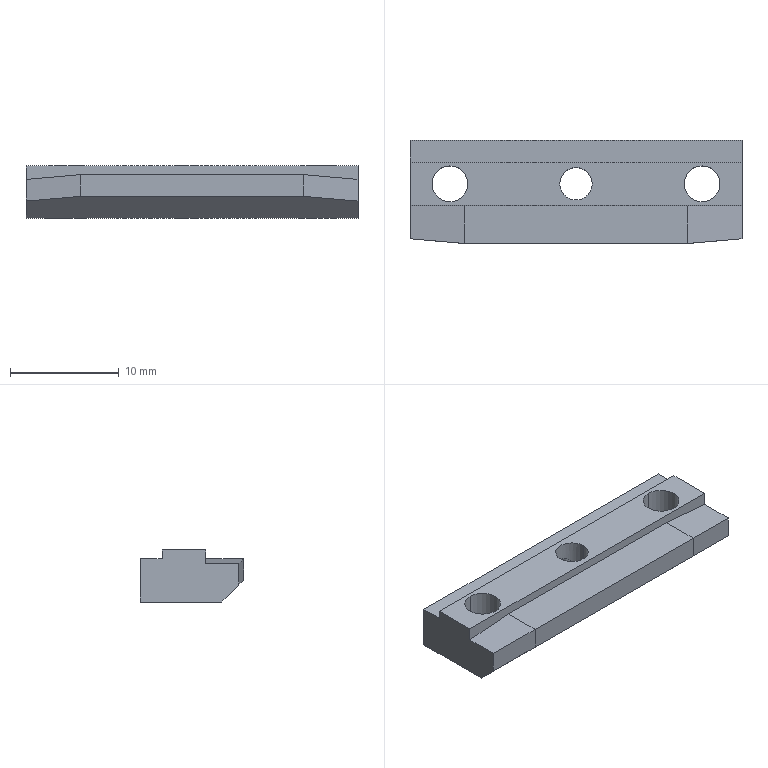Part | NX | 1 solid | 29 faces | box 30.6 x 9.5 x 4.8 mm | volume 1058 mm3 | plane 15 | cylinder 8 | cone 6 | commonest cylinder face diameters 3.3 x4 2.5 x2 3 x2
STEP:
#1=CARTESIAN_POINT('',(-174.8,180.7,-95.7));
#2=VERTEX_POINT('',#1);
#3=CARTESIAN_POINT('',(-174.8,176.706,-95.7));
#4=VERTEX_POINT('',#3);
#5=CARTESIAN_POINT('',(-174.8,178.513,-95.7));
#6=DIRECTION('',(0.,-1.,0.));
#7=VECTOR('',#6,1000.);
#8=LINE('',#5,#7);
#9=EDGE_CURVE('',#2,#4,#8,.T.);
#10=ORIENTED_EDGE('',*,*,#9,.T.);
#11=CARTESIAN_POINT('',(-144.2,176.706,-95.7));
#12=VERTEX_POINT('',#11);
#13=CARTESIAN_POINT('',(-175.,176.706,-95.7));
#14=DIRECTION('',(-1.,0.,0.));
#15=VECTOR('',#14,1000.);
#16=LINE('',#13,#15);
#17=EDGE_CURVE('',#12,#4,#16,.T.);
#18=ORIENTED_EDGE('',*,*,#17,.F.);
#19=CARTESIAN_POINT('',(-144.2,180.7,-95.7));
#20=VERTEX_POINT('',#19);
#21=CARTESIAN_POINT('',(-144.2,178.513,-95.7));
#22=DIRECTION('',(0.,-1.,0.));
#23=VECTOR('',#22,1000.);
#24=LINE('',#21,#23);
#25=EDGE_CURVE('',#20,#12,#24,.T.);
#26=ORIENTED_EDGE('',*,*,#25,.F.);
#27=CARTESIAN_POINT('',(-175.,180.7,-95.7));
#28=DIRECTION('',(1.,0.,0.));
#29=VECTOR('',#28,1000.);
#30=LINE('',#27,#29);
#31=EDGE_CURVE('',#2,#20,#30,.T.);
#32=ORIENTED_EDGE('',*,*,#31,.F.);
#33=EDGE_LOOP('',(#10,#18,#26,#32));
#34=FACE_BOUND('',#33,.T.);
#35=CARTESIAN_POINT('',(-147.875,177.05,-95.7));
#36=VERTEX_POINT('',#35);
#37=CARTESIAN_POINT('',(-147.875,180.35,-95.7));
#38=VERTEX_POINT('',#37);
#39=CARTESIAN_POINT('',(-147.875,178.7,-95.7));
#40=DIRECTION('',(0.,0.,-1.));
#41=DIRECTION('',(0.,1.,0.));
#42=AXIS2_PLACEMENT_3D('',#39,#40,#41);
#43=CIRCLE('',#42,1.65);
#44=EDGE_CURVE('',#36,#38,#43,.T.);
#45=ORIENTED_EDGE('',*,*,#44,.T.);
#46=CARTESIAN_POINT('',(-147.875,178.7,-95.7));
#47=DIRECTION('',(0.,0.,-1.));
#48=DIRECTION('',(0.,1.,0.));
#49=AXIS2_PLACEMENT_3D('',#46,#47,#48);
#50=CIRCLE('',#49,1.65);
#51=EDGE_CURVE('',#38,#36,#50,.T.);
#52=ORIENTED_EDGE('',*,*,#51,.T.);
#53=EDGE_LOOP('',(#45,#52));
#54=FACE_BOUND('',#53,.T.);
#55=CARTESIAN_POINT('',(-171.125,177.05,-95.7));
#56=VERTEX_POINT('',#55);
#57=CARTESIAN_POINT('',(-171.125,180.35,-95.7));
#58=VERTEX_POINT('',#57);
#59=CARTESIAN_POINT('',(-171.125,178.7,-95.7));
#60=DIRECTION('',(0.,0.,-1.));
#61=DIRECTION('',(0.,1.,0.));
#62=AXIS2_PLACEMENT_3D('',#59,#60,#61);
#63=CIRCLE('',#62,1.65);
#64=EDGE_CURVE('',#56,#58,#63,.T.);
#65=ORIENTED_EDGE('',*,*,#64,.T.);
#66=CARTESIAN_POINT('',(-171.125,178.7,-95.7));
#67=DIRECTION('',(0.,0.,-1.));
#68=DIRECTION('',(0.,1.,0.));
#69=AXIS2_PLACEMENT_3D('',#66,#67,#68);
#70=CIRCLE('',#69,1.65);
#71=EDGE_CURVE('',#58,#56,#70,.T.);
#72=ORIENTED_EDGE('',*,*,#71,.T.);
#73=EDGE_LOOP('',(#65,#72));
#74=FACE_BOUND('',#73,.T.);
#75=CARTESIAN_POINT('',(-158.,178.7,-95.7));
#76=VERTEX_POINT('',#75);
#77=CARTESIAN_POINT('',(-161.,178.7,-95.7));
#78=VERTEX_POINT('',#77);
#79=CARTESIAN_POINT('',(-159.5,178.7,-95.7));
#80=DIRECTION('',(0.,0.,-1.));
#81=DIRECTION('',(-1.,0.,0.));
#82=AXIS2_PLACEMENT_3D('',#79,#80,#81);
#83=CIRCLE('',#82,1.5);
#84=EDGE_CURVE('',#76,#78,#83,.T.);
#85=ORIENTED_EDGE('',*,*,#84,.T.);
#86=CARTESIAN_POINT('',(-159.5,178.7,-95.7));
#87=DIRECTION('',(0.,0.,-1.));
#88=DIRECTION('',(-1.,0.,0.));
#89=AXIS2_PLACEMENT_3D('',#86,#87,#88);
#90=CIRCLE('',#89,1.5);
#91=EDGE_CURVE('',#78,#76,#90,.T.);
#92=ORIENTED_EDGE('',*,*,#91,.T.);
#93=EDGE_LOOP('',(#85,#92));
#94=FACE_BOUND('',#93,.T.);
#95=CARTESIAN_POINT('',(-175.,176.707,-95.7));
#96=DIRECTION('',(0.,0.,1.));
#97=DIRECTION('',(1.,0.,0.));
#98=AXIS2_PLACEMENT_3D('',#95,#96,#97);
#99=PLANE('',#98);
#100=ADVANCED_FACE('',(#34,#54,#74,#94),#99,.T.);
#101=CARTESIAN_POINT('',(-174.8,176.697,-96.937));
#102=VERTEX_POINT('',#101);
#103=CARTESIAN_POINT('',(-174.8,176.744,-90.15));
#104=DIRECTION('',(0.,-0.007004,-1.));
#105=VECTOR('',#104,1000.);
#106=LINE('',#103,#105);
#107=EDGE_CURVE('',#4,#102,#106,.T.);
#108=ORIENTED_EDGE('',*,*,#107,.T.);
#109=CARTESIAN_POINT('',(-169.8,176.7,-96.5));
#110=VERTEX_POINT('',#109);
#111=CARTESIAN_POINT('',(-175.,176.697,-96.955));
#112=DIRECTION('',(-0.9962,-0.0006105,-0.08716));
#113=VECTOR('',#112,1000.);
#114=LINE('',#111,#113);
#115=EDGE_CURVE('',#110,#102,#114,.T.);
#116=ORIENTED_EDGE('',*,*,#115,.F.);
#117=CARTESIAN_POINT('',(-149.2,176.7,-96.5));
#118=VERTEX_POINT('',#117);
#119=CARTESIAN_POINT('',(-175.,176.7,-96.5));
#120=DIRECTION('',(1.,0.,0.));
#121=VECTOR('',#120,1000.);
#122=LINE('',#119,#121);
#123=EDGE_CURVE('',#110,#118,#122,.T.);
#124=ORIENTED_EDGE('',*,*,#123,.T.);
#125=CARTESIAN_POINT('',(-144.2,176.697,-96.937));
#126=VERTEX_POINT('',#125);
#127=CARTESIAN_POINT('',(-175.,176.716,-94.243));
#128=DIRECTION('',(0.9962,-0.0006105,-0.08716));
#129=VECTOR('',#128,1000.);
#130=LINE('',#127,#129);
#131=EDGE_CURVE('',#118,#126,#130,.T.);
#132=ORIENTED_EDGE('',*,*,#131,.T.);
#133=CARTESIAN_POINT('',(-144.2,176.744,-90.15));
#134=DIRECTION('',(0.,-0.007004,-1.));
#135=VECTOR('',#134,1000.);
#136=LINE('',#133,#135);
#137=EDGE_CURVE('',#12,#126,#136,.T.);
#138=ORIENTED_EDGE('',*,*,#137,.F.);
#139=ORIENTED_EDGE('',*,*,#17,.T.);
#140=EDGE_LOOP('',(#108,#116,#124,#132,#138,#139));
#141=FACE_BOUND('',#140,.T.);
#142=CARTESIAN_POINT('',(-175.,176.7,-96.5));
#143=DIRECTION('',(0.,-1.,0.007004));
#144=DIRECTION('',(-1.,0.,0.));
#145=AXIS2_PLACEMENT_3D('',#142,#143,#144);
#146=PLANE('',#145);
#147=ADVANCED_FACE('',(#141),#146,.T.);
#148=CARTESIAN_POINT('',(-169.8,173.2,-96.5));
#149=VERTEX_POINT('',#148);
#150=CARTESIAN_POINT('',(-169.8,174.95,-96.5));
#151=DIRECTION('',(0.,-1.,0.));
#152=VECTOR('',#151,1000.);
#153=LINE('',#150,#152);
#154=EDGE_CURVE('',#110,#149,#153,.T.);
#155=ORIENTED_EDGE('',*,*,#154,.T.);
#156=CARTESIAN_POINT('',(-149.2,173.2,-96.5));
#157=VERTEX_POINT('',#156);
#158=CARTESIAN_POINT('',(-175.,173.2,-96.5));
#159=DIRECTION('',(1.,0.,0.));
#160=VECTOR('',#159,1000.);
#161=LINE('',#158,#160);
#162=EDGE_CURVE('',#149,#157,#161,.T.);
#163=ORIENTED_EDGE('',*,*,#162,.T.);
#164=CARTESIAN_POINT('',(-149.2,174.95,-96.5));
#165=DIRECTION('',(0.,-1.,0.));
#166=VECTOR('',#165,1000.);
#167=LINE('',#164,#166);
#168=EDGE_CURVE('',#118,#157,#167,.T.);
#169=ORIENTED_EDGE('',*,*,#168,.F.);
#170=ORIENTED_EDGE('',*,*,#123,.F.);
#171=EDGE_LOOP('',(#155,#163,#169,#170));
#172=FACE_BOUND('',#171,.T.);
#173=CARTESIAN_POINT('',(-175.,174.7,-96.5));
#174=DIRECTION('',(0.,0.,1.));
#175=DIRECTION('',(1.,0.,0.));
#176=AXIS2_PLACEMENT_3D('',#173,#174,#175);
#177=PLANE('',#176);
#178=ADVANCED_FACE('',(#172),#177,.T.);
#179=CARTESIAN_POINT('',(-149.2,173.2,-98.5));
#180=VERTEX_POINT('',#179);
#181=CARTESIAN_POINT('',(-169.8,173.2,-98.5));
#182=VERTEX_POINT('',#181);
#183=CARTESIAN_POINT('',(-175.,173.2,-98.5));
#184=DIRECTION('',(-1.,0.,0.));
#185=VECTOR('',#184,1000.);
#186=LINE('',#183,#185);
#187=EDGE_CURVE('',#180,#182,#186,.T.);
#188=ORIENTED_EDGE('',*,*,#187,.F.);
#189=CARTESIAN_POINT('',(-149.2,173.2,-97.5));
#190=DIRECTION('',(0.,0.,-1.));
#191=VECTOR('',#190,1000.);
#192=LINE('',#189,#191);
#193=EDGE_CURVE('',#157,#180,#192,.T.);
#194=ORIENTED_EDGE('',*,*,#193,.F.);
#195=ORIENTED_EDGE('',*,*,#162,.F.);
#196=CARTESIAN_POINT('',(-169.8,173.2,-97.5));
#197=DIRECTION('',(0.,0.,-1.));
#198=VECTOR('',#197,1000.);
#199=LINE('',#196,#198);
#200=EDGE_CURVE('',#149,#182,#199,.T.);
#201=ORIENTED_EDGE('',*,*,#200,.T.);
#202=EDGE_LOOP('',(#188,#194,#195,#201));
#203=FACE_BOUND('',#202,.T.);
#204=CARTESIAN_POINT('',(-175.,173.2,-100.5));
#205=DIRECTION('',(0.,-1.,0.));
#206=DIRECTION('',(-1.,0.,0.));
#207=AXIS2_PLACEMENT_3D('',#204,#205,#206);
#208=PLANE('',#207);
#209=ADVANCED_FACE('',(#203),#208,.T.);
#210=CARTESIAN_POINT('',(-174.8,175.2,-100.5));
#211=VERTEX_POINT('',#210);
#212=CARTESIAN_POINT('',(-174.8,182.7,-100.5));
#213=VERTEX_POINT('',#212);
#214=CARTESIAN_POINT('',(-174.8,178.513,-100.5));
#215=DIRECTION('',(0.,1.,0.));
#216=VECTOR('',#215,1000.);
#217=LINE('',#214,#216);
#218=EDGE_CURVE('',#211,#213,#217,.T.);
#219=ORIENTED_EDGE('',*,*,#218,.T.);
#220=CARTESIAN_POINT('',(-144.2,182.7,-100.5));
#221=VERTEX_POINT('',#220);
#222=CARTESIAN_POINT('',(-175.,182.7,-100.5));
#223=DIRECTION('',(1.,0.,0.));
#224=VECTOR('',#223,1000.);
#225=LINE('',#222,#224);
#226=EDGE_CURVE('',#213,#221,#225,.T.);
#227=ORIENTED_EDGE('',*,*,#226,.T.);
#228=CARTESIAN_POINT('',(-144.2,175.2,-100.5));
#229=VERTEX_POINT('',#228);
#230=CARTESIAN_POINT('',(-144.2,178.513,-100.5));
#231=DIRECTION('',(0.,1.,0.));
#232=VECTOR('',#231,1000.);
#233=LINE('',#230,#232);
#234=EDGE_CURVE('',#229,#221,#233,.T.);
#235=ORIENTED_EDGE('',*,*,#234,.F.);
#236=CARTESIAN_POINT('',(-175.,175.2,-100.5));
#237=DIRECTION('',(-1.,0.,0.));
#238=VECTOR('',#237,1000.);
#239=LINE('',#236,#238);
#240=EDGE_CURVE('',#229,#211,#239,.T.);
#241=ORIENTED_EDGE('',*,*,#240,.T.);
#242=EDGE_LOOP('',(#219,#227,#235,#241));
#243=FACE_BOUND('',#242,.T.);
#244=CARTESIAN_POINT('',(-158.,178.7,-100.5));
#245=VERTEX_POINT('',#244);
#246=CARTESIAN_POINT('',(-161.,178.7,-100.5));
#247=VERTEX_POINT('',#246);
#248=CARTESIAN_POINT('',(-159.5,178.7,-100.5));
#249=DIRECTION('',(0.,0.,-1.));
#250=DIRECTION('',(-1.,0.,0.));
#251=AXIS2_PLACEMENT_3D('',#248,#249,#250);
#252=CIRCLE('',#251,1.5);
#253=EDGE_CURVE('',#245,#247,#252,.T.);
#254=ORIENTED_EDGE('',*,*,#253,.F.);
#255=CARTESIAN_POINT('',(-159.5,178.7,-100.5));
#256=DIRECTION('',(0.,0.,-1.));
#257=DIRECTION('',(-1.,0.,0.));
#258=AXIS2_PLACEMENT_3D('',#255,#256,#257);
#259=CIRCLE('',#258,1.5);
#260=EDGE_CURVE('',#247,#245,#259,.T.);
#261=ORIENTED_EDGE('',*,*,#260,.F.);
#262=EDGE_LOOP('',(#254,#261));
#263=FACE_BOUND('',#262,.T.);
#264=CARTESIAN_POINT('',(-171.125,176.85,-100.5));
#265=VERTEX_POINT('',#264);
#266=CARTESIAN_POINT('',(-171.125,180.55,-100.5));
#267=VERTEX_POINT('',#266);
#268=CARTESIAN_POINT('',(-171.125,178.7,-100.5));
#269=DIRECTION('',(0.,0.,-1.));
#270=DIRECTION('',(0.,1.,0.));
#271=AXIS2_PLACEMENT_3D('',#268,#269,#270);
#272=CIRCLE('',#271,1.85);
#273=EDGE_CURVE('',#265,#267,#272,.T.);
#274=ORIENTED_EDGE('',*,*,#273,.F.);
#275=CARTESIAN_POINT('',(-171.125,178.7,-100.5));
#276=DIRECTION('',(0.,0.,-1.));
#277=DIRECTION('',(0.,1.,0.));
#278=AXIS2_PLACEMENT_3D('',#275,#276,#277);
#279=CIRCLE('',#278,1.85);
#280=EDGE_CURVE('',#267,#265,#279,.T.);
#281=ORIENTED_EDGE('',*,*,#280,.F.);
#282=EDGE_LOOP('',(#274,#281));
#283=FACE_BOUND('',#282,.T.);
#284=CARTESIAN_POINT('',(-147.875,176.85,-100.5));
#285=VERTEX_POINT('',#284);
#286=CARTESIAN_POINT('',(-147.875,180.55,-100.5));
#287=VERTEX_POINT('',#286);
#288=CARTESIAN_POINT('',(-147.875,178.7,-100.5));
#289=DIRECTION('',(0.,0.,-1.));
#290=DIRECTION('',(0.,1.,0.));
#291=AXIS2_PLACEMENT_3D('',#288,#289,#290);
#292=CIRCLE('',#291,1.85);
#293=EDGE_CURVE('',#285,#287,#292,.T.);
#294=ORIENTED_EDGE('',*,*,#293,.F.);
#295=CARTESIAN_POINT('',(-147.875,178.7,-100.5));
#296=DIRECTION('',(0.,0.,-1.));
#297=DIRECTION('',(0.,1.,0.));
#298=AXIS2_PLACEMENT_3D('',#295,#296,#297);
#299=CIRCLE('',#298,1.85);
#300=EDGE_CURVE('',#287,#285,#299,.T.);
#301=ORIENTED_EDGE('',*,*,#300,.F.);
#302=EDGE_LOOP('',(#294,#301));
#303=FACE_BOUND('',#302,.T.);
#304=CARTESIAN_POINT('',(-175.,182.7,-100.5));
#305=DIRECTION('',(0.,0.,-1.));
#306=DIRECTION('',(-1.,0.,0.));
#307=AXIS2_PLACEMENT_3D('',#304,#305,#306);
#308=PLANE('',#307);
#309=ADVANCED_FACE('',(#243,#263,#283,#303),#308,.T.);
#310=CARTESIAN_POINT('',(-174.8,182.7,-96.5));
#311=VERTEX_POINT('',#310);
#312=CARTESIAN_POINT('',(-174.8,182.7,-90.15));
#313=DIRECTION('',(0.,0.,1.));
#314=VECTOR('',#313,1000.);
#315=LINE('',#312,#314);
#316=EDGE_CURVE('',#213,#311,#315,.T.);
#317=ORIENTED_EDGE('',*,*,#316,.T.);
#318=CARTESIAN_POINT('',(-144.2,182.7,-96.5));
#319=VERTEX_POINT('',#318);
#320=CARTESIAN_POINT('',(-175.,182.7,-96.5));
#321=DIRECTION('',(1.,0.,0.));
#322=VECTOR('',#321,1000.);
#323=LINE('',#320,#322);
#324=EDGE_CURVE('',#311,#319,#323,.T.);
#325=ORIENTED_EDGE('',*,*,#324,.T.);
#326=CARTESIAN_POINT('',(-144.2,182.7,-90.15));
#327=DIRECTION('',(0.,0.,1.));
#328=VECTOR('',#327,1000.);
#329=LINE('',#326,#328);
#330=EDGE_CURVE('',#221,#319,#329,.T.);
#331=ORIENTED_EDGE('',*,*,#330,.F.);
#332=ORIENTED_EDGE('',*,*,#226,.F.);
#333=EDGE_LOOP('',(#317,#325,#331,#332));
#334=FACE_BOUND('',#333,.T.);
#335=CARTESIAN_POINT('',(-159.5,182.7,-100.2));
#336=VERTEX_POINT('',#335);
#337=CARTESIAN_POINT('',(-159.5,182.7,-96.8));
#338=VERTEX_POINT('',#337);
#339=CARTESIAN_POINT('',(-159.5,182.7,-98.5));
#340=DIRECTION('',(0.,1.,0.));
#341=DIRECTION('',(0.,0.,1.));
#342=AXIS2_PLACEMENT_3D('',#339,#340,#341);
#343=CIRCLE('',#342,1.7);
#344=EDGE_CURVE('',#336,#338,#343,.T.);
#345=ORIENTED_EDGE('',*,*,#344,.F.);
#346=CARTESIAN_POINT('',(-159.5,182.7,-98.5));
#347=DIRECTION('',(0.,1.,0.));
#348=DIRECTION('',(0.,0.,1.));
#349=AXIS2_PLACEMENT_3D('',#346,#347,#348);
#350=CIRCLE('',#349,1.7);
#351=EDGE_CURVE('',#338,#336,#350,.T.);
#352=ORIENTED_EDGE('',*,*,#351,.F.);
#353=EDGE_LOOP('',(#345,#352));
#354=FACE_BOUND('',#353,.T.);
#355=CARTESIAN_POINT('',(-175.,182.7,-96.5));
#356=DIRECTION('',(0.,1.,0.));
#357=DIRECTION('',(1.,0.,0.));
#358=AXIS2_PLACEMENT_3D('',#355,#356,#357);
#359=PLANE('',#358);
#360=ADVANCED_FACE('',(#334,#354),#359,.T.);
#361=CARTESIAN_POINT('',(-174.8,180.7,-96.5));
#362=VERTEX_POINT('',#361);
#363=CARTESIAN_POINT('',(-174.8,178.513,-96.5));
#364=DIRECTION('',(0.,-1.,0.));
#365=VECTOR('',#364,1000.);
#366=LINE('',#363,#365);
#367=EDGE_CURVE('',#311,#362,#366,.T.);
#368=ORIENTED_EDGE('',*,*,#367,.T.);
#369=CARTESIAN_POINT('',(-144.2,180.7,-96.5));
#370=VERTEX_POINT('',#369);
#371=CARTESIAN_POINT('',(-175.,180.7,-96.5));
#372=DIRECTION('',(1.,0.,0.));
#373=VECTOR('',#372,1000.);
#374=LINE('',#371,#373);
#375=EDGE_CURVE('',#362,#370,#374,.T.);
#376=ORIENTED_EDGE('',*,*,#375,.T.);
#377=CARTESIAN_POINT('',(-144.2,178.513,-96.5));
#378=DIRECTION('',(0.,-1.,0.));
#379=VECTOR('',#378,1000.);
#380=LINE('',#377,#379);
#381=EDGE_CURVE('',#319,#370,#380,.T.);
#382=ORIENTED_EDGE('',*,*,#381,.F.);
#383=ORIENTED_EDGE('',*,*,#324,.F.);
#384=EDGE_LOOP('',(#368,#376,#382,#383));
#385=FACE_BOUND('',#384,.T.);
#386=CARTESIAN_POINT('',(-175.,180.7,-96.5));
#387=DIRECTION('',(0.,0.,1.));
#388=DIRECTION('',(1.,0.,0.));
#389=AXIS2_PLACEMENT_3D('',#386,#387,#388);
#390=PLANE('',#389);
#391=ADVANCED_FACE('',(#385),#390,.T.);
#392=CARTESIAN_POINT('',(-174.8,180.7,-90.15));
#393=DIRECTION('',(0.,0.,1.));
#394=VECTOR('',#393,1000.);
#395=LINE('',#392,#394);
#396=EDGE_CURVE('',#362,#2,#395,.T.);
#397=ORIENTED_EDGE('',*,*,#396,.T.);
#398=ORIENTED_EDGE('',*,*,#31,.T.);
#399=CARTESIAN_POINT('',(-144.2,180.7,-90.15));
#400=DIRECTION('',(0.,0.,1.));
#401=VECTOR('',#400,1000.);
#402=LINE('',#399,#401);
#403=EDGE_CURVE('',#370,#20,#402,.T.);
#404=ORIENTED_EDGE('',*,*,#403,.F.);
#405=ORIENTED_EDGE('',*,*,#375,.F.);
#406=EDGE_LOOP('',(#397,#398,#404,#405));
#407=FACE_BOUND('',#406,.T.);
#408=CARTESIAN_POINT('',(-175.,180.7,-95.5));
#409=DIRECTION('',(0.,1.,0.));
#410=DIRECTION('',(1.,0.,0.));
#411=AXIS2_PLACEMENT_3D('',#408,#409,#410);
#412=PLANE('',#411);
#413=ADVANCED_FACE('',(#407),#412,.T.);
#414=CARTESIAN_POINT('',(-171.125,177.05,-100.3));
#415=VERTEX_POINT('',#414);
#416=CARTESIAN_POINT('',(-171.125,180.35,-100.3));
#417=VERTEX_POINT('',#416);
#418=CARTESIAN_POINT('',(-171.125,178.7,-100.3));
#419=DIRECTION('',(0.,0.,-1.));
#420=DIRECTION('',(0.,1.,0.));
#421=AXIS2_PLACEMENT_3D('',#418,#419,#420);
#422=CIRCLE('',#421,1.65);
#423=EDGE_CURVE('',#415,#417,#422,.T.);
#424=ORIENTED_EDGE('',*,*,#423,.T.);
#425=CARTESIAN_POINT('',(-171.125,180.35,-100.5));
#426=DIRECTION('',(0.,0.,-1.));
#427=VECTOR('',#426,1000.);
#428=LINE('',#425,#427);
#429=EDGE_CURVE('',#417,#58,#428,.F.);
#430=ORIENTED_EDGE('',*,*,#429,.T.);
#431=ORIENTED_EDGE('',*,*,#64,.F.);
#432=CARTESIAN_POINT('',(-171.125,177.05,-100.5));
#433=DIRECTION('',(0.,0.,-1.));
#434=VECTOR('',#433,1000.);
#435=LINE('',#432,#434);
#436=EDGE_CURVE('',#415,#56,#435,.F.);
#437=ORIENTED_EDGE('',*,*,#436,.F.);
#438=EDGE_LOOP('',(#424,#430,#431,#437));
#439=FACE_BOUND('',#438,.T.);
#440=CARTESIAN_POINT('',(-171.125,178.7,-100.5));
#441=DIRECTION('',(0.,0.,-1.));
#442=DIRECTION('',(0.,1.,0.));
#443=AXIS2_PLACEMENT_3D('',#440,#441,#442);
#444=CYLINDRICAL_SURFACE('',#443,1.65);
#445=ADVANCED_FACE('',(#439),#444,.F.);
#446=ORIENTED_EDGE('',*,*,#423,.F.);
#447=CARTESIAN_POINT('',(-171.125,177.05,-100.3));
#448=DIRECTION('',(0.,-0.7071,-0.7071));
#449=VECTOR('',#448,1000.);
#450=LINE('',#447,#449);
#451=EDGE_CURVE('',#265,#415,#450,.F.);
#452=ORIENTED_EDGE('',*,*,#451,.F.);
#453=ORIENTED_EDGE('',*,*,#273,.T.);
#454=CARTESIAN_POINT('',(-171.125,180.35,-100.3));
#455=DIRECTION('',(0.,0.7071,-0.7071));
#456=VECTOR('',#455,1000.);
#457=LINE('',#454,#456);
#458=EDGE_CURVE('',#267,#417,#457,.F.);
#459=ORIENTED_EDGE('',*,*,#458,.T.);
#460=EDGE_LOOP('',(#446,#452,#453,#459));
#461=FACE_BOUND('',#460,.T.);
#462=CARTESIAN_POINT('',(-171.125,178.7,-100.3));
#463=DIRECTION('',(0.,0.,-1.));
#464=DIRECTION('',(0.,1.,0.));
#465=AXIS2_PLACEMENT_3D('',#462,#463,#464);
#466=CONICAL_SURFACE('',#465,1.65,0.7854);
#467=ADVANCED_FACE('',(#461),#466,.F.);
#468=CARTESIAN_POINT('',(-147.875,177.05,-100.3));
#469=VERTEX_POINT('',#468);
#470=CARTESIAN_POINT('',(-147.875,180.35,-100.3));
#471=VERTEX_POINT('',#470);
#472=CARTESIAN_POINT('',(-147.875,178.7,-100.3));
#473=DIRECTION('',(0.,0.,-1.));
#474=DIRECTION('',(0.,1.,0.));
#475=AXIS2_PLACEMENT_3D('',#472,#473,#474);
#476=CIRCLE('',#475,1.65);
#477=EDGE_CURVE('',#469,#471,#476,.T.);
#478=ORIENTED_EDGE('',*,*,#477,.T.);
#479=CARTESIAN_POINT('',(-147.875,180.35,-100.5));
#480=DIRECTION('',(0.,0.,-1.));
#481=VECTOR('',#480,1000.);
#482=LINE('',#479,#481);
#483=EDGE_CURVE('',#471,#38,#482,.F.);
#484=ORIENTED_EDGE('',*,*,#483,.T.);
#485=ORIENTED_EDGE('',*,*,#44,.F.);
#486=CARTESIAN_POINT('',(-147.875,177.05,-100.5));
#487=DIRECTION('',(0.,0.,-1.));
#488=VECTOR('',#487,1000.);
#489=LINE('',#486,#488);
#490=EDGE_CURVE('',#469,#36,#489,.F.);
#491=ORIENTED_EDGE('',*,*,#490,.F.);
#492=EDGE_LOOP('',(#478,#484,#485,#491));
#493=FACE_BOUND('',#492,.T.);
#494=CARTESIAN_POINT('',(-147.875,178.7,-100.5));
#495=DIRECTION('',(0.,0.,-1.));
#496=DIRECTION('',(0.,1.,0.));
#497=AXIS2_PLACEMENT_3D('',#494,#495,#496);
#498=CYLINDRICAL_SURFACE('',#497,1.65);
#499=ADVANCED_FACE('',(#493),#498,.F.);
#500=ORIENTED_EDGE('',*,*,#477,.F.);
#501=CARTESIAN_POINT('',(-147.875,177.05,-100.3));
#502=DIRECTION('',(0.,-0.7071,-0.7071));
#503=VECTOR('',#502,1000.);
#504=LINE('',#501,#503);
#505=EDGE_CURVE('',#285,#469,#504,.F.);
#506=ORIENTED_EDGE('',*,*,#505,.F.);
#507=ORIENTED_EDGE('',*,*,#293,.T.);
#508=CARTESIAN_POINT('',(-147.875,180.35,-100.3));
#509=DIRECTION('',(0.,0.7071,-0.7071));
#510=VECTOR('',#509,1000.);
#511=LINE('',#508,#510);
#512=EDGE_CURVE('',#287,#471,#511,.F.);
#513=ORIENTED_EDGE('',*,*,#512,.T.);
#514=EDGE_LOOP('',(#500,#506,#507,#513));
#515=FACE_BOUND('',#514,.T.);
#516=CARTESIAN_POINT('',(-147.875,178.7,-100.3));
#517=DIRECTION('',(0.,0.,-1.));
#518=DIRECTION('',(0.,1.,0.));
#519=AXIS2_PLACEMENT_3D('',#516,#517,#518);
#520=CONICAL_SURFACE('',#519,1.65,0.7854);
#521=ADVANCED_FACE('',(#515),#520,.F.);
#522=ORIENTED_EDGE('',*,*,#84,.F.);
#523=CARTESIAN_POINT('',(-158.,178.7,-95.22));
#524=DIRECTION('',(0.,0.,-1.));
#525=VECTOR('',#524,1000.);
#526=LINE('',#523,#525);
#527=EDGE_CURVE('',#245,#76,#526,.F.);
#528=ORIENTED_EDGE('',*,*,#527,.F.);
#529=ORIENTED_EDGE('',*,*,#253,.T.);
#530=CARTESIAN_POINT('',(-161.,178.7,-95.22));
#531=DIRECTION('',(0.,0.,-1.));
#532=VECTOR('',#531,1000.);
#533=LINE('',#530,#532);
#534=EDGE_CURVE('',#247,#78,#533,.F.);
#535=ORIENTED_EDGE('',*,*,#534,.T.);
#536=EDGE_LOOP('',(#522,#528,#529,#535));
#537=FACE_BOUND('',#536,.T.);
#538=CARTESIAN_POINT('',(-159.5,178.7,-95.22));
#539=DIRECTION('',(0.,0.,-1.));
#540=DIRECTION('',(-1.,0.,0.));
#541=AXIS2_PLACEMENT_3D('',#538,#539,#540);
#542=CYLINDRICAL_SURFACE('',#541,1.5);
#543=ADVANCED_FACE('',(#537),#542,.F.);
#544=ORIENTED_EDGE('',*,*,#187,.T.);
#545=CARTESIAN_POINT('',(-174.8,173.637,-98.937));
#546=VERTEX_POINT('',#545);
#547=CARTESIAN_POINT('',(-175.,173.655,-98.955));
#548=DIRECTION('',(0.9924,-0.08683,0.08683));
#549=VECTOR('',#548,1000.);
#550=LINE('',#547,#549);
#551=EDGE_CURVE('',#546,#182,#550,.T.);
#552=ORIENTED_EDGE('',*,*,#551,.F.);
#553=CARTESIAN_POINT('',(-174.8,164.85,-90.15));
#554=DIRECTION('',(0.,-0.7071,0.7071));
#555=VECTOR('',#554,1000.);
#556=LINE('',#553,#555);
#557=EDGE_CURVE('',#211,#546,#556,.T.);
#558=ORIENTED_EDGE('',*,*,#557,.F.);
#559=ORIENTED_EDGE('',*,*,#240,.F.);
#560=CARTESIAN_POINT('',(-144.2,173.637,-98.937));
#561=VERTEX_POINT('',#560);
#562=CARTESIAN_POINT('',(-144.2,164.85,-90.15));
#563=DIRECTION('',(0.,-0.7071,0.7071));
#564=VECTOR('',#563,1000.);
#565=LINE('',#562,#564);
#566=EDGE_CURVE('',#229,#561,#565,.T.);
#567=ORIENTED_EDGE('',*,*,#566,.T.);
#568=CARTESIAN_POINT('',(-175.,170.943,-96.243));
#569=DIRECTION('',(-0.9924,-0.08683,0.08683));
#570=VECTOR('',#569,1000.);
#571=LINE('',#568,#570);
#572=EDGE_CURVE('',#561,#180,#571,.T.);
#573=ORIENTED_EDGE('',*,*,#572,.T.);
#574=EDGE_LOOP('',(#544,#552,#558,#559,#567,#573));
#575=FACE_BOUND('',#574,.T.);
#576=CARTESIAN_POINT('',(-159.5,174.2,-99.5));
#577=DIRECTION('',(0.,0.7071,0.7071));
#578=DIRECTION('',(1.,0.,0.));
#579=AXIS2_PLACEMENT_3D('',#576,#577,#578);
#580=PLANE('',#579);
#581=ADVANCED_FACE('',(#575),#580,.F.);
#582=CARTESIAN_POINT('',(-159.5,182.44,-99.75));
#583=VERTEX_POINT('',#582);
#584=CARTESIAN_POINT('',(-159.5,182.44,-97.25));
#585=VERTEX_POINT('',#584);
#586=CARTESIAN_POINT('',(-159.5,182.44,-98.5));
#587=DIRECTION('',(0.,1.,0.));
#588=DIRECTION('',(0.,0.,1.));
#589=AXIS2_PLACEMENT_3D('',#586,#587,#588);
#590=CIRCLE('',#589,1.25);
#591=EDGE_CURVE('',#583,#585,#590,.T.);
#592=ORIENTED_EDGE('',*,*,#591,.T.);
#593=CARTESIAN_POINT('',(-159.5,180.2,-97.25));
#594=VERTEX_POINT('',#593);
#595=CARTESIAN_POINT('',(-159.5,182.7,-97.25));
#596=DIRECTION('',(0.,1.,0.));
#597=VECTOR('',#596,1000.);
#598=LINE('',#595,#597);
#599=EDGE_CURVE('',#594,#585,#598,.T.);
#600=ORIENTED_EDGE('',*,*,#599,.F.);
#601=CARTESIAN_POINT('',(-160.75,179.529,-98.5));
#602=VERTEX_POINT('',#601);
#603=CARTESIAN_POINT('',(-160.75,179.529,-98.5));
#604=CARTESIAN_POINT('',(-160.75,179.529,-98.489));
#605=CARTESIAN_POINT('',(-160.75,179.529,-98.478));
#606=CARTESIAN_POINT('',(-160.75,179.53,-98.467));
#607=CARTESIAN_POINT('',(-160.749,179.53,-98.457));
#608=CARTESIAN_POINT('',(-160.749,179.531,-98.446));
#609=CARTESIAN_POINT('',(-160.748,179.532,-98.435));
#610=CARTESIAN_POINT('',(-160.748,179.533,-98.424));
#611=CARTESIAN_POINT('',(-160.747,179.534,-98.413));
#612=CARTESIAN_POINT('',(-160.746,179.535,-98.402));
#613=CARTESIAN_POINT('',(-160.745,179.536,-98.391));
#614=CARTESIAN_POINT('',(-160.744,179.538,-98.381));
#615=CARTESIAN_POINT('',(-160.743,179.539,-98.37));
#616=CARTESIAN_POINT('',(-160.741,179.543,-98.348));
#617=CARTESIAN_POINT('',(-160.738,179.547,-98.327));
#618=CARTESIAN_POINT('',(-160.735,179.552,-98.306));
#619=CARTESIAN_POINT('',(-160.731,179.556,-98.285));
#620=CARTESIAN_POINT('',(-160.728,179.562,-98.264));
#621=CARTESIAN_POINT('',(-160.723,179.568,-98.243));
#622=CARTESIAN_POINT('',(-160.715,179.58,-98.203));
#623=CARTESIAN_POINT('',(-160.704,179.594,-98.163));
#624=CARTESIAN_POINT('',(-160.692,179.61,-98.124));
#625=CARTESIAN_POINT('',(-160.686,179.618,-98.105));
#626=CARTESIAN_POINT('',(-160.679,179.627,-98.085));
#627=CARTESIAN_POINT('',(-160.672,179.636,-98.067));
#628=CARTESIAN_POINT('',(-160.666,179.644,-98.048));
#629=CARTESIAN_POINT('',(-160.658,179.653,-98.029));
#630=CARTESIAN_POINT('',(-160.65,179.663,-98.011));
#631=CARTESIAN_POINT('',(-160.643,179.672,-97.993));
#632=CARTESIAN_POINT('',(-160.635,179.681,-97.975));
#633=CARTESIAN_POINT('',(-160.626,179.691,-97.957));
#634=CARTESIAN_POINT('',(-160.618,179.701,-97.94));
#635=CARTESIAN_POINT('',(-160.609,179.71,-97.922));
#636=CARTESIAN_POINT('',(-160.599,179.72,-97.905));
#637=CARTESIAN_POINT('',(-160.59,179.73,-97.888));
#638=CARTESIAN_POINT('',(-160.581,179.74,-97.871));
#639=CARTESIAN_POINT('',(-160.571,179.751,-97.855));
#640=CARTESIAN_POINT('',(-160.561,179.761,-97.838));
#641=CARTESIAN_POINT('',(-160.55,179.771,-97.822));
#642=CARTESIAN_POINT('',(-160.54,179.781,-97.806));
#643=CARTESIAN_POINT('',(-160.529,179.792,-97.79));
#644=CARTESIAN_POINT('',(-160.518,179.802,-97.774));
#645=CARTESIAN_POINT('',(-160.506,179.812,-97.759));
#646=CARTESIAN_POINT('',(-160.495,179.823,-97.743));
#647=CARTESIAN_POINT('',(-160.483,179.833,-97.728));
#648=CARTESIAN_POINT('',(-160.471,179.843,-97.713));
#649=CARTESIAN_POINT('',(-160.447,179.864,-97.683));
#650=CARTESIAN_POINT('',(-160.421,179.885,-97.654));
#651=CARTESIAN_POINT('',(-160.394,179.905,-97.626));
#652=CARTESIAN_POINT('',(-160.366,179.925,-97.598));
#653=CARTESIAN_POINT('',(-160.338,179.945,-97.572));
#654=CARTESIAN_POINT('',(-160.308,179.964,-97.546));
#655=CARTESIAN_POINT('',(-160.293,179.973,-97.534));
#656=CARTESIAN_POINT('',(-160.278,179.983,-97.521));
#657=CARTESIAN_POINT('',(-160.262,179.992,-97.509));
#658=CARTESIAN_POINT('',(-160.246,180.001,-97.497));
#659=CARTESIAN_POINT('',(-160.23,180.01,-97.485));
#660=CARTESIAN_POINT('',(-160.214,180.019,-97.474));
#661=CARTESIAN_POINT('',(-160.198,180.028,-97.463));
#662=CARTESIAN_POINT('',(-160.181,180.037,-97.451));
#663=CARTESIAN_POINT('',(-160.164,180.045,-97.441));
#664=CARTESIAN_POINT('',(-160.146,180.054,-97.43));
#665=CARTESIAN_POINT('',(-160.129,180.062,-97.42));
#666=CARTESIAN_POINT('',(-160.111,180.07,-97.41));
#667=CARTESIAN_POINT('',(-160.093,180.078,-97.4));
#668=CARTESIAN_POINT('',(-160.075,180.085,-97.39));
#669=CARTESIAN_POINT('',(-160.057,180.093,-97.381));
#670=CARTESIAN_POINT('',(-160.038,180.1,-97.372));
#671=CARTESIAN_POINT('',(-160.019,180.107,-97.363));
#672=CARTESIAN_POINT('',(-160.,180.114,-97.355));
#673=CARTESIAN_POINT('',(-159.962,180.128,-97.338));
#674=CARTESIAN_POINT('',(-159.923,180.14,-97.323));
#675=CARTESIAN_POINT('',(-159.883,180.15,-97.31));
#676=CARTESIAN_POINT('',(-159.863,180.156,-97.304));
#677=CARTESIAN_POINT('',(-159.842,180.161,-97.298));
#678=CARTESIAN_POINT('',(-159.822,180.165,-97.292));
#679=CARTESIAN_POINT('',(-159.801,180.17,-97.287));
#680=CARTESIAN_POINT('',(-159.78,180.174,-97.282));
#681=CARTESIAN_POINT('',(-159.759,180.177,-97.277));
#682=CARTESIAN_POINT('',(-159.738,180.181,-97.273));
#683=CARTESIAN_POINT('',(-159.716,180.184,-97.269));
#684=CARTESIAN_POINT('',(-159.695,180.187,-97.265));
#685=CARTESIAN_POINT('',(-159.674,180.19,-97.262));
#686=CARTESIAN_POINT('',(-159.652,180.192,-97.259));
#687=CARTESIAN_POINT('',(-159.63,180.194,-97.257));
#688=CARTESIAN_POINT('',(-159.609,180.196,-97.255));
#689=CARTESIAN_POINT('',(-159.587,180.198,-97.253));
#690=CARTESIAN_POINT('',(-159.565,180.199,-97.252));
#691=CARTESIAN_POINT('',(-159.544,180.2,-97.251));
#692=CARTESIAN_POINT('',(-159.522,180.2,-97.25));
#693=CARTESIAN_POINT('',(-159.5,180.2,-97.25));
#694=B_SPLINE_CURVE_WITH_KNOTS('',3,(#603,#604,#605,#606,#607,#608,#609,#610,#611,#612,#613,#614,#615,#616,#617,#618,#619,#620,#621,#622,#623,#624,#625,#626,#627,#628,#629,#630,#631,#632,#633,#634,#635,#636,#637,#638,#639,#640,#641,#642,#643,#644,#645,#646,#647,#648,#649,#650,#651,#652,#653,#654,#655,#656,#657,#658,#659,#660,#661,#662,#663,#664,#665,#666,#667,#668,#669,#670,#671,#672,#673,#674,#675,#676,#677,#678,#679,#680,#681,#682,#683,#684,#685,#686,#687,#688,#689,#690,#691,#692,#693),.UNSPECIFIED.,.F.,.F.,(4,3,3,3,3,3,3,3,3,3,3,3,3,3,3,3,3,3,3,3,3,3,3,3,3,3,3,3,3,3,4),(0.,0.03265,0.06539,0.0982,0.1311,0.1968,0.2623,0.393,0.4586,0.5242,0.5897,0.655,0.7205,0.7861,0.8518,0.9176,1.049,1.18,1.245,1.311,1.377,1.443,1.508,1.574,1.705,1.77,1.836,1.902,1.967,2.033,2.098),.UNSPECIFIED.);
#695=EDGE_CURVE('',#602,#594,#694,.T.);
#696=ORIENTED_EDGE('',*,*,#695,.F.);
#697=CARTESIAN_POINT('',(-159.5,180.2,-99.75));
#698=VERTEX_POINT('',#697);
#699=CARTESIAN_POINT('',(-159.5,180.2,-99.75));
#700=CARTESIAN_POINT('',(-159.522,180.2,-99.75));
#701=CARTESIAN_POINT('',(-159.544,180.2,-99.749));
#702=CARTESIAN_POINT('',(-159.566,180.199,-99.748));
#703=CARTESIAN_POINT('',(-159.587,180.198,-99.747));
#704=CARTESIAN_POINT('',(-159.609,180.196,-99.745));
#705=CARTESIAN_POINT('',(-159.631,180.194,-99.743));
#706=CARTESIAN_POINT('',(-159.652,180.192,-99.741));
#707=CARTESIAN_POINT('',(-159.674,180.19,-99.738));
#708=CARTESIAN_POINT('',(-159.695,180.187,-99.735));
#709=CARTESIAN_POINT('',(-159.716,180.184,-99.731));
#710=CARTESIAN_POINT('',(-159.738,180.181,-99.727));
#711=CARTESIAN_POINT('',(-159.759,180.178,-99.723));
#712=CARTESIAN_POINT('',(-159.78,180.174,-99.718));
#713=CARTESIAN_POINT('',(-159.801,180.17,-99.713));
#714=CARTESIAN_POINT('',(-159.822,180.165,-99.708));
#715=CARTESIAN_POINT('',(-159.842,180.161,-99.702));
#716=CARTESIAN_POINT('',(-159.863,180.156,-99.696));
#717=CARTESIAN_POINT('',(-159.883,180.15,-99.69));
#718=CARTESIAN_POINT('',(-159.903,180.145,-99.683));
#719=CARTESIAN_POINT('',(-159.923,180.139,-99.676));
#720=CARTESIAN_POINT('',(-159.943,180.133,-99.669));
#721=CARTESIAN_POINT('',(-159.962,180.127,-99.662));
#722=CARTESIAN_POINT('',(-159.981,180.121,-99.654));
#723=CARTESIAN_POINT('',(-160.,180.114,-99.645));
#724=CARTESIAN_POINT('',(-160.019,180.107,-99.637));
#725=CARTESIAN_POINT('',(-160.038,180.1,-99.628));
#726=CARTESIAN_POINT('',(-160.057,180.093,-99.619));
#727=CARTESIAN_POINT('',(-160.075,180.086,-99.61));
#728=CARTESIAN_POINT('',(-160.093,180.078,-99.601));
#729=CARTESIAN_POINT('',(-160.111,180.07,-99.591));
#730=CARTESIAN_POINT('',(-160.129,180.062,-99.581));
#731=CARTESIAN_POINT('',(-160.146,180.054,-99.57));
#732=CARTESIAN_POINT('',(-160.163,180.045,-99.559));
#733=CARTESIAN_POINT('',(-160.181,180.037,-99.549));
#734=CARTESIAN_POINT('',(-160.197,180.028,-99.538));
#735=CARTESIAN_POINT('',(-160.214,180.019,-99.526));
#736=CARTESIAN_POINT('',(-160.23,180.01,-99.515));
#737=CARTESIAN_POINT('',(-160.246,180.001,-99.503));
#738=CARTESIAN_POINT('',(-160.262,179.992,-99.491));
#739=CARTESIAN_POINT('',(-160.278,179.983,-99.479));
#740=CARTESIAN_POINT('',(-160.293,179.973,-99.467));
#741=CARTESIAN_POINT('',(-160.308,179.964,-99.454));
#742=CARTESIAN_POINT('',(-160.338,179.945,-99.429));
#743=CARTESIAN_POINT('',(-160.366,179.925,-99.402));
#744=CARTESIAN_POINT('',(-160.393,179.905,-99.374));
#745=CARTESIAN_POINT('',(-160.421,179.885,-99.347));
#746=CARTESIAN_POINT('',(-160.446,179.864,-99.318));
#747=CARTESIAN_POINT('',(-160.471,179.844,-99.288));
#748=CARTESIAN_POINT('',(-160.483,179.833,-99.273));
#749=CARTESIAN_POINT('',(-160.495,179.823,-99.257));
#750=CARTESIAN_POINT('',(-160.506,179.812,-99.242));
#751=CARTESIAN_POINT('',(-160.518,179.802,-99.226));
#752=CARTESIAN_POINT('',(-160.529,179.792,-99.21));
#753=CARTESIAN_POINT('',(-160.539,179.781,-99.194));
#754=CARTESIAN_POINT('',(-160.55,179.771,-99.178));
#755=CARTESIAN_POINT('',(-160.561,179.761,-99.162));
#756=CARTESIAN_POINT('',(-160.571,179.751,-99.145));
#757=CARTESIAN_POINT('',(-160.581,179.74,-99.129));
#758=CARTESIAN_POINT('',(-160.59,179.73,-99.112));
#759=CARTESIAN_POINT('',(-160.599,179.72,-99.095));
#760=CARTESIAN_POINT('',(-160.609,179.71,-99.078));
#761=CARTESIAN_POINT('',(-160.618,179.701,-99.06));
#762=CARTESIAN_POINT('',(-160.626,179.691,-99.043));
#763=CARTESIAN_POINT('',(-160.634,179.681,-99.025));
#764=CARTESIAN_POINT('',(-160.643,179.672,-99.007));
#765=CARTESIAN_POINT('',(-160.65,179.663,-98.989));
#766=CARTESIAN_POINT('',(-160.658,179.653,-98.971));
#767=CARTESIAN_POINT('',(-160.665,179.644,-98.952));
#768=CARTESIAN_POINT('',(-160.672,179.636,-98.934));
#769=CARTESIAN_POINT('',(-160.679,179.627,-98.915));
#770=CARTESIAN_POINT('',(-160.686,179.619,-98.896));
#771=CARTESIAN_POINT('',(-160.692,179.611,-98.876));
#772=CARTESIAN_POINT('',(-160.704,179.594,-98.837));
#773=CARTESIAN_POINT('',(-160.715,179.58,-98.797));
#774=CARTESIAN_POINT('',(-160.723,179.568,-98.757));
#775=CARTESIAN_POINT('',(-160.728,179.562,-98.736));
#776=CARTESIAN_POINT('',(-160.731,179.556,-98.715));
#777=CARTESIAN_POINT('',(-160.735,179.552,-98.694));
#778=CARTESIAN_POINT('',(-160.738,179.547,-98.673));
#779=CARTESIAN_POINT('',(-160.741,179.543,-98.652));
#780=CARTESIAN_POINT('',(-160.743,179.539,-98.63));
#781=CARTESIAN_POINT('',(-160.744,179.538,-98.62));
#782=CARTESIAN_POINT('',(-160.745,179.536,-98.609));
#783=CARTESIAN_POINT('',(-160.746,179.535,-98.598));
#784=CARTESIAN_POINT('',(-160.747,179.534,-98.587));
#785=CARTESIAN_POINT('',(-160.748,179.533,-98.576));
#786=CARTESIAN_POINT('',(-160.748,179.532,-98.565));
#787=CARTESIAN_POINT('',(-160.749,179.531,-98.555));
#788=CARTESIAN_POINT('',(-160.749,179.53,-98.544));
#789=CARTESIAN_POINT('',(-160.75,179.53,-98.533));
#790=CARTESIAN_POINT('',(-160.75,179.529,-98.522));
#791=CARTESIAN_POINT('',(-160.75,179.529,-98.511));
#792=CARTESIAN_POINT('',(-160.75,179.529,-98.5));
#793=B_SPLINE_CURVE_WITH_KNOTS('',3,(#699,#700,#701,#702,#703,#704,#705,#706,#707,#708,#709,#710,#711,#712,#713,#714,#715,#716,#717,#718,#719,#720,#721,#722,#723,#724,#725,#726,#727,#728,#729,#730,#731,#732,#733,#734,#735,#736,#737,#738,#739,#740,#741,#742,#743,#744,#745,#746,#747,#748,#749,#750,#751,#752,#753,#754,#755,#756,#757,#758,#759,#760,#761,#762,#763,#764,#765,#766,#767,#768,#769,#770,#771,#772,#773,#774,#775,#776,#777,#778,#779,#780,#781,#782,#783,#784,#785,#786,#787,#788,#789,#790,#791,#792),.UNSPECIFIED.,.F.,.F.,(4,3,3,3,3,3,3,3,3,3,3,3,3,3,3,3,3,3,3,3,3,3,3,3,3,3,3,3,3,3,3,4),(0.,0.06563,0.131,0.1964,0.262,0.3277,0.3933,0.4588,0.5241,0.5896,0.6553,0.721,0.7868,0.8524,0.9178,1.049,1.18,1.246,1.312,1.377,1.443,1.508,1.574,1.639,1.705,1.836,1.901,1.967,2.,2.033,2.065,2.098),.UNSPECIFIED.);
#794=EDGE_CURVE('',#698,#602,#793,.T.);
#795=ORIENTED_EDGE('',*,*,#794,.F.);
#796=CARTESIAN_POINT('',(-159.5,182.7,-99.75));
#797=DIRECTION('',(0.,1.,0.));
#798=VECTOR('',#797,1000.);
#799=LINE('',#796,#798);
#800=EDGE_CURVE('',#698,#583,#799,.T.);
#801=ORIENTED_EDGE('',*,*,#800,.T.);
#802=EDGE_LOOP('',(#592,#600,#696,#795,#801));
#803=FACE_BOUND('',#802,.T.);
#804=CARTESIAN_POINT('',(-159.5,182.7,-98.5));
#805=DIRECTION('',(0.,1.,0.));
#806=DIRECTION('',(0.,0.,1.));
#807=AXIS2_PLACEMENT_3D('',#804,#805,#806);
#808=CYLINDRICAL_SURFACE('',#807,1.25);
#809=ADVANCED_FACE('',(#803),#808,.F.);
#810=ORIENTED_EDGE('',*,*,#591,.F.);
#811=CARTESIAN_POINT('',(-159.5,182.44,-99.75));
#812=DIRECTION('',(0.,0.5,-0.866));
#813=VECTOR('',#812,1000.);
#814=LINE('',#811,#813);
#815=EDGE_CURVE('',#583,#336,#814,.T.);
#816=ORIENTED_EDGE('',*,*,#815,.T.);
#817=ORIENTED_EDGE('',*,*,#344,.T.);
#818=CARTESIAN_POINT('',(-159.5,182.44,-97.25));
#819=DIRECTION('',(0.,0.5,0.866));
#820=VECTOR('',#819,1000.);
#821=LINE('',#818,#820);
#822=EDGE_CURVE('',#585,#338,#821,.T.);
#823=ORIENTED_EDGE('',*,*,#822,.F.);
#824=EDGE_LOOP('',(#810,#816,#817,#823));
#825=FACE_BOUND('',#824,.T.);
#826=CARTESIAN_POINT('',(-159.5,182.44,-98.5));
#827=DIRECTION('',(0.,1.,0.));
#828=DIRECTION('',(0.,0.,1.));
#829=AXIS2_PLACEMENT_3D('',#826,#827,#828);
#830=CONICAL_SURFACE('',#829,1.25,1.047);
#831=ADVANCED_FACE('',(#825),#830,.F.);
#832=ORIENTED_EDGE('',*,*,#436,.T.);
#833=ORIENTED_EDGE('',*,*,#71,.F.);
#834=ORIENTED_EDGE('',*,*,#429,.F.);
#835=CARTESIAN_POINT('',(-171.125,178.7,-100.3));
#836=DIRECTION('',(0.,0.,-1.));
#837=DIRECTION('',(0.,1.,0.));
#838=AXIS2_PLACEMENT_3D('',#835,#836,#837);
#839=CIRCLE('',#838,1.65);
#840=EDGE_CURVE('',#417,#415,#839,.T.);
#841=ORIENTED_EDGE('',*,*,#840,.T.);
#842=EDGE_LOOP('',(#832,#833,#834,#841));
#843=FACE_BOUND('',#842,.T.);
#844=CARTESIAN_POINT('',(-171.125,178.7,-100.5));
#845=DIRECTION('',(0.,0.,-1.));
#846=DIRECTION('',(0.,1.,0.));
#847=AXIS2_PLACEMENT_3D('',#844,#845,#846);
#848=CYLINDRICAL_SURFACE('',#847,1.65);
#849=ADVANCED_FACE('',(#843),#848,.F.);
#850=ORIENTED_EDGE('',*,*,#451,.T.);
#851=ORIENTED_EDGE('',*,*,#840,.F.);
#852=ORIENTED_EDGE('',*,*,#458,.F.);
#853=ORIENTED_EDGE('',*,*,#280,.T.);
#854=EDGE_LOOP('',(#850,#851,#852,#853));
#855=FACE_BOUND('',#854,.T.);
#856=CARTESIAN_POINT('',(-171.125,178.7,-100.3));
#857=DIRECTION('',(0.,0.,-1.));
#858=DIRECTION('',(0.,1.,0.));
#859=AXIS2_PLACEMENT_3D('',#856,#857,#858);
#860=CONICAL_SURFACE('',#859,1.65,0.7854);
#861=ADVANCED_FACE('',(#855),#860,.F.);
#862=ORIENTED_EDGE('',*,*,#534,.F.);
#863=ORIENTED_EDGE('',*,*,#260,.T.);
#864=ORIENTED_EDGE('',*,*,#527,.T.);
#865=ORIENTED_EDGE('',*,*,#91,.F.);
#866=EDGE_LOOP('',(#862,#863,#864,#865));
#867=FACE_BOUND('',#866,.T.);
#868=ORIENTED_EDGE('',*,*,#794,.T.);
#869=ORIENTED_EDGE('',*,*,#695,.T.);
#870=CARTESIAN_POINT('',(-159.5,180.2,-97.25));
#871=CARTESIAN_POINT('',(-159.472,180.2,-97.25));
#872=CARTESIAN_POINT('',(-159.444,180.199,-97.251));
#873=CARTESIAN_POINT('',(-159.415,180.198,-97.253));
#874=CARTESIAN_POINT('',(-159.4,180.197,-97.254));
#875=CARTESIAN_POINT('',(-159.385,180.196,-97.255));
#876=CARTESIAN_POINT('',(-159.37,180.194,-97.257));
#877=CARTESIAN_POINT('',(-159.355,180.193,-97.258));
#878=CARTESIAN_POINT('',(-159.34,180.192,-97.26));
#879=CARTESIAN_POINT('',(-159.325,180.19,-97.262));
#880=CARTESIAN_POINT('',(-159.31,180.188,-97.264));
#881=CARTESIAN_POINT('',(-159.295,180.186,-97.267));
#882=CARTESIAN_POINT('',(-159.28,180.184,-97.269));
#883=CARTESIAN_POINT('',(-159.266,180.182,-97.272));
#884=CARTESIAN_POINT('',(-159.251,180.179,-97.275));
#885=CARTESIAN_POINT('',(-159.236,180.177,-97.278));
#886=CARTESIAN_POINT('',(-159.207,180.171,-97.284));
#887=CARTESIAN_POINT('',(-159.179,180.165,-97.292));
#888=CARTESIAN_POINT('',(-159.15,180.159,-97.3));
#889=CARTESIAN_POINT('',(-159.122,180.152,-97.308));
#890=CARTESIAN_POINT('',(-159.094,180.144,-97.317));
#891=CARTESIAN_POINT('',(-159.066,180.136,-97.328));
#892=CARTESIAN_POINT('',(-159.039,180.128,-97.338));
#893=CARTESIAN_POINT('',(-159.012,180.119,-97.349));
#894=CARTESIAN_POINT('',(-158.986,180.109,-97.361));
#895=CARTESIAN_POINT('',(-158.96,180.1,-97.373));
#896=CARTESIAN_POINT('',(-158.934,180.089,-97.385));
#897=CARTESIAN_POINT('',(-158.909,180.079,-97.399));
#898=CARTESIAN_POINT('',(-158.896,180.073,-97.405));
#899=CARTESIAN_POINT('',(-158.884,180.068,-97.412));
#900=CARTESIAN_POINT('',(-158.872,180.062,-97.419));
#901=CARTESIAN_POINT('',(-158.86,180.057,-97.426));
#902=CARTESIAN_POINT('',(-158.848,180.051,-97.433));
#903=CARTESIAN_POINT('',(-158.836,180.045,-97.441));
#904=CARTESIAN_POINT('',(-158.812,180.033,-97.456));
#905=CARTESIAN_POINT('',(-158.789,180.021,-97.471));
#906=CARTESIAN_POINT('',(-158.767,180.009,-97.487));
#907=CARTESIAN_POINT('',(-158.742,179.995,-97.506));
#908=CARTESIAN_POINT('',(-158.718,179.98,-97.525));
#909=CARTESIAN_POINT('',(-158.694,179.965,-97.544));
#910=CARTESIAN_POINT('',(-158.671,179.95,-97.564));
#911=CARTESIAN_POINT('',(-158.649,179.935,-97.584));
#912=CARTESIAN_POINT('',(-158.627,179.92,-97.605));
#913=CARTESIAN_POINT('',(-158.605,179.904,-97.626));
#914=CARTESIAN_POINT('',(-158.585,179.889,-97.648));
#915=CARTESIAN_POINT('',(-158.565,179.873,-97.671));
#916=CARTESIAN_POINT('',(-158.555,179.865,-97.682));
#917=CARTESIAN_POINT('',(-158.545,179.857,-97.693));
#918=CARTESIAN_POINT('',(-158.536,179.849,-97.705));
#919=CARTESIAN_POINT('',(-158.526,179.841,-97.716));
#920=CARTESIAN_POINT('',(-158.517,179.833,-97.728));
#921=CARTESIAN_POINT('',(-158.508,179.825,-97.739));
#922=CARTESIAN_POINT('',(-158.49,179.809,-97.763));
#923=CARTESIAN_POINT('',(-158.473,179.793,-97.787));
#924=CARTESIAN_POINT('',(-158.456,179.777,-97.813));
#925=CARTESIAN_POINT('',(-158.44,179.761,-97.838));
#926=CARTESIAN_POINT('',(-158.424,179.745,-97.863));
#927=CARTESIAN_POINT('',(-158.409,179.73,-97.889));
#928=CARTESIAN_POINT('',(-158.395,179.714,-97.916));
#929=CARTESIAN_POINT('',(-158.381,179.699,-97.943));
#930=CARTESIAN_POINT('',(-158.368,179.684,-97.97));
#931=CARTESIAN_POINT('',(-158.355,179.669,-97.998));
#932=CARTESIAN_POINT('',(-158.343,179.655,-98.026));
#933=CARTESIAN_POINT('',(-158.332,179.641,-98.055));
#934=CARTESIAN_POINT('',(-158.326,179.633,-98.072));
#935=CARTESIAN_POINT('',(-158.32,179.625,-98.089));
#936=CARTESIAN_POINT('',(-158.314,179.618,-98.106));
#937=CARTESIAN_POINT('',(-158.308,179.611,-98.123));
#938=CARTESIAN_POINT('',(-158.303,179.604,-98.141));
#939=CARTESIAN_POINT('',(-158.298,179.597,-98.158));
#940=CARTESIAN_POINT('',(-158.293,179.59,-98.176));
#941=CARTESIAN_POINT('',(-158.288,179.584,-98.194));
#942=CARTESIAN_POINT('',(-158.284,179.578,-98.213));
#943=CARTESIAN_POINT('',(-158.279,179.572,-98.231));
#944=CARTESIAN_POINT('',(-158.275,179.566,-98.249));
#945=CARTESIAN_POINT('',(-158.272,179.561,-98.268));
#946=CARTESIAN_POINT('',(-158.268,179.556,-98.287));
#947=CARTESIAN_POINT('',(-158.265,179.551,-98.306));
#948=CARTESIAN_POINT('',(-158.262,179.548,-98.325));
#949=CARTESIAN_POINT('',(-158.26,179.544,-98.344));
#950=CARTESIAN_POINT('',(-158.257,179.54,-98.363));
#951=CARTESIAN_POINT('',(-158.256,179.537,-98.382));
#952=CARTESIAN_POINT('',(-158.254,179.535,-98.401));
#953=CARTESIAN_POINT('',(-158.252,179.533,-98.421));
#954=CARTESIAN_POINT('',(-158.251,179.531,-98.441));
#955=CARTESIAN_POINT('',(-158.25,179.53,-98.46));
#956=CARTESIAN_POINT('',(-158.25,179.529,-98.48));
#957=CARTESIAN_POINT('',(-158.25,179.529,-98.5));
#958=CARTESIAN_POINT('',(-158.25,179.529,-98.519));
#959=CARTESIAN_POINT('',(-158.25,179.53,-98.539));
#960=CARTESIAN_POINT('',(-158.251,179.531,-98.559));
#961=CARTESIAN_POINT('',(-158.252,179.533,-98.578));
#962=CARTESIAN_POINT('',(-158.254,179.535,-98.598));
#963=CARTESIAN_POINT('',(-158.256,179.537,-98.617));
#964=CARTESIAN_POINT('',(-158.257,179.54,-98.637));
#965=CARTESIAN_POINT('',(-158.26,179.543,-98.656));
#966=CARTESIAN_POINT('',(-158.262,179.547,-98.675));
#967=CARTESIAN_POINT('',(-158.265,179.551,-98.694));
#968=CARTESIAN_POINT('',(-158.268,179.556,-98.713));
#969=CARTESIAN_POINT('',(-158.272,179.561,-98.731));
#970=CARTESIAN_POINT('',(-158.275,179.566,-98.75));
#971=CARTESIAN_POINT('',(-158.279,179.571,-98.769));
#972=CARTESIAN_POINT('',(-158.283,179.577,-98.787));
#973=CARTESIAN_POINT('',(-158.288,179.583,-98.805));
#974=CARTESIAN_POINT('',(-158.292,179.59,-98.823));
#975=CARTESIAN_POINT('',(-158.297,179.597,-98.841));
#976=CARTESIAN_POINT('',(-158.302,179.603,-98.859));
#977=CARTESIAN_POINT('',(-158.308,179.61,-98.876));
#978=CARTESIAN_POINT('',(-158.314,179.618,-98.894));
#979=CARTESIAN_POINT('',(-158.319,179.625,-98.911));
#980=CARTESIAN_POINT('',(-158.325,179.633,-98.928));
#981=CARTESIAN_POINT('',(-158.332,179.641,-98.944));
#982=CARTESIAN_POINT('',(-158.343,179.654,-98.973));
#983=CARTESIAN_POINT('',(-158.355,179.669,-99.002));
#984=CARTESIAN_POINT('',(-158.367,179.684,-99.029));
#985=CARTESIAN_POINT('',(-158.38,179.698,-99.057));
#986=CARTESIAN_POINT('',(-158.394,179.714,-99.084));
#987=CARTESIAN_POINT('',(-158.409,179.729,-99.11));
#988=CARTESIAN_POINT('',(-158.424,179.745,-99.136));
#989=CARTESIAN_POINT('',(-158.439,179.761,-99.162));
#990=CARTESIAN_POINT('',(-158.456,179.777,-99.187));
#991=CARTESIAN_POINT('',(-158.472,179.793,-99.212));
#992=CARTESIAN_POINT('',(-158.489,179.809,-99.236));
#993=CARTESIAN_POINT('',(-158.507,179.825,-99.26));
#994=CARTESIAN_POINT('',(-158.516,179.833,-99.272));
#995=CARTESIAN_POINT('',(-158.526,179.841,-99.283));
#996=CARTESIAN_POINT('',(-158.535,179.849,-99.295));
#997=CARTESIAN_POINT('',(-158.545,179.856,-99.306));
#998=CARTESIAN_POINT('',(-158.554,179.864,-99.318));
#999=CARTESIAN_POINT('',(-158.564,179.872,-99.329));
#1000=CARTESIAN_POINT('',(-158.584,179.888,-99.351));
#1001=CARTESIAN_POINT('',(-158.605,179.904,-99.373));
#1002=CARTESIAN_POINT('',(-158.626,179.919,-99.394));
#1003=CARTESIAN_POINT('',(-158.648,179.935,-99.415));
#1004=CARTESIAN_POINT('',(-158.671,179.95,-99.436));
#1005=CARTESIAN_POINT('',(-158.694,179.965,-99.455));
#1006=CARTESIAN_POINT('',(-158.717,179.98,-99.475));
#1007=CARTESIAN_POINT('',(-158.741,179.994,-99.494));
#1008=CARTESIAN_POINT('',(-158.767,180.008,-99.512));
#1009=CARTESIAN_POINT('',(-158.789,180.021,-99.528));
#1010=CARTESIAN_POINT('',(-158.812,180.033,-99.544));
#1011=CARTESIAN_POINT('',(-158.836,180.045,-99.559));
#1012=CARTESIAN_POINT('',(-158.859,180.057,-99.574));
#1013=CARTESIAN_POINT('',(-158.884,180.068,-99.588));
#1014=CARTESIAN_POINT('',(-158.908,180.078,-99.601));
#1015=CARTESIAN_POINT('',(-158.933,180.089,-99.615));
#1016=CARTESIAN_POINT('',(-158.959,180.099,-99.627));
#1017=CARTESIAN_POINT('',(-158.985,180.109,-99.639));
#1018=CARTESIAN_POINT('',(-159.011,180.118,-99.651));
#1019=CARTESIAN_POINT('',(-159.038,180.127,-99.662));
#1020=CARTESIAN_POINT('',(-159.066,180.136,-99.672));
#1021=CARTESIAN_POINT('',(-159.093,180.144,-99.682));
#1022=CARTESIAN_POINT('',(-159.121,180.152,-99.692));
#1023=CARTESIAN_POINT('',(-159.15,180.159,-99.7));
#1024=CARTESIAN_POINT('',(-159.178,180.165,-99.708));
#1025=CARTESIAN_POINT('',(-159.207,180.171,-99.716));
#1026=CARTESIAN_POINT('',(-159.236,180.177,-99.722));
#1027=CARTESIAN_POINT('',(-159.251,180.179,-99.725));
#1028=CARTESIAN_POINT('',(-159.266,180.182,-99.728));
#1029=CARTESIAN_POINT('',(-159.28,180.184,-99.731));
#1030=CARTESIAN_POINT('',(-159.295,180.186,-99.733));
#1031=CARTESIAN_POINT('',(-159.31,180.188,-99.736));
#1032=CARTESIAN_POINT('',(-159.325,180.19,-99.738));
#1033=CARTESIAN_POINT('',(-159.339,180.191,-99.74));
#1034=CARTESIAN_POINT('',(-159.354,180.193,-99.742));
#1035=CARTESIAN_POINT('',(-159.369,180.194,-99.743));
#1036=CARTESIAN_POINT('',(-159.385,180.196,-99.745));
#1037=CARTESIAN_POINT('',(-159.4,180.197,-99.746));
#1038=CARTESIAN_POINT('',(-159.415,180.198,-99.747));
#1039=CARTESIAN_POINT('',(-159.443,180.199,-99.749));
#1040=CARTESIAN_POINT('',(-159.472,180.2,-99.75));
#1041=CARTESIAN_POINT('',(-159.5,180.2,-99.75));
#1042=B_SPLINE_CURVE_WITH_KNOTS('',3,(#870,#871,#872,#873,#874,#875,#876,#877,#878,#879,#880,#881,#882,#883,#884,#885,#886,#887,#888,#889,#890,#891,#892,#893,#894,#895,#896,#897,#898,#899,#900,#901,#902,#903,#904,#905,#906,#907,#908,#909,#910,#911,#912,#913,#914,#915,#916,#917,#918,#919,#920,#921,#922,#923,#924,#925,#926,#927,#928,#929,#930,#931,#932,#933,#934,#935,#936,#937,#938,#939,#940,#941,#942,#943,#944,#945,#946,#947,#948,#949,#950,#951,#952,#953,#954,#955,#956,#957,#958,#959,#960,#961,#962,#963,#964,#965,#966,#967,#968,#969,#970,#971,#972,#973,#974,#975,#976,#977,#978,#979,#980,#981,#982,#983,#984,#985,#986,#987,#988,#989,#990,#991,#992,#993,#994,#995,#996,#997,#998,#999,#1000,#1001,#1002,#1003,#1004,#1005,#1006,#1007,#1008,#1009,#1010,#1011,#1012,#1013,#1014,#1015,#1016,#1017,#1018,#1019,#1020,#1021,#1022,#1023,#1024,#1025,#1026,#1027,#1028,#1029,#1030,#1031,#1032,#1033,#1034,#1035,#1036,#1037,#1038,#1039,#1040,#1041),.UNSPECIFIED.,.F.,.F.,(4,3,3,3,3,3,3,3,3,3,3,3,3,3,3,3,3,3,3,3,3,3,3,3,3,3,3,3,3,3,3,3,3,3,3,3,3,3,3,3,3,3,3,3,3,3,3,3,3,3,3,3,3,3,3,3,3,4),(0.,0.08477,0.1304,0.176,0.2215,0.2669,0.3577,0.4488,0.54,0.631,0.6763,0.7217,0.8127,0.9145,1.016,1.118,1.169,1.219,1.321,1.423,1.524,1.626,1.685,1.744,1.803,1.862,1.921,1.98,2.038,2.098,2.157,2.216,2.275,2.334,2.393,2.452,2.511,2.57,2.671,2.772,2.874,2.976,3.027,3.077,3.179,3.281,3.383,3.474,3.565,3.655,3.747,3.838,3.929,3.974,4.02,4.065,4.111,4.196),.UNSPECIFIED.);
#1043=EDGE_CURVE('',#594,#698,#1042,.T.);
#1044=ORIENTED_EDGE('',*,*,#1043,.T.);
#1045=EDGE_LOOP('',(#868,#869,#1044));
#1046=FACE_BOUND('',#1045,.T.);
#1047=CARTESIAN_POINT('',(-159.5,178.7,-95.22));
#1048=DIRECTION('',(0.,0.,-1.));
#1049=DIRECTION('',(-1.,0.,0.));
#1050=AXIS2_PLACEMENT_3D('',#1047,#1048,#1049);
#1051=CYLINDRICAL_SURFACE('',#1050,1.5);
#1052=ADVANCED_FACE('',(#867,#1046),#1051,.F.);
#1053=ORIENTED_EDGE('',*,*,#599,.T.);
#1054=CARTESIAN_POINT('',(-159.5,182.44,-98.5));
#1055=DIRECTION('',(0.,1.,0.));
#1056=DIRECTION('',(0.,0.,1.));
#1057=AXIS2_PLACEMENT_3D('',#1054,#1055,#1056);
#1058=CIRCLE('',#1057,1.25);
#1059=EDGE_CURVE('',#585,#583,#1058,.T.);
#1060=ORIENTED_EDGE('',*,*,#1059,.T.);
#1061=ORIENTED_EDGE('',*,*,#800,.F.);
#1062=ORIENTED_EDGE('',*,*,#1043,.F.);
#1063=EDGE_LOOP('',(#1053,#1060,#1061,#1062));
#1064=FACE_BOUND('',#1063,.T.);
#1065=CARTESIAN_POINT('',(-159.5,182.7,-98.5));
#1066=DIRECTION('',(0.,1.,0.));
#1067=DIRECTION('',(0.,0.,1.));
#1068=AXIS2_PLACEMENT_3D('',#1065,#1066,#1067);
#1069=CYLINDRICAL_SURFACE('',#1068,1.25);
#1070=ADVANCED_FACE('',(#1064),#1069,.F.);
#1071=ORIENTED_EDGE('',*,*,#505,.T.);
#1072=CARTESIAN_POINT('',(-147.875,178.7,-100.3));
#1073=DIRECTION('',(0.,0.,-1.));
#1074=DIRECTION('',(0.,1.,0.));
#1075=AXIS2_PLACEMENT_3D('',#1072,#1073,#1074);
#1076=CIRCLE('',#1075,1.65);
#1077=EDGE_CURVE('',#471,#469,#1076,.T.);
#1078=ORIENTED_EDGE('',*,*,#1077,.F.);
#1079=ORIENTED_EDGE('',*,*,#512,.F.);
#1080=ORIENTED_EDGE('',*,*,#300,.T.);
#1081=EDGE_LOOP('',(#1071,#1078,#1079,#1080));
#1082=FACE_BOUND('',#1081,.T.);
#1083=CARTESIAN_POINT('',(-147.875,178.7,-100.3));
#1084=DIRECTION('',(0.,0.,-1.));
#1085=DIRECTION('',(0.,1.,0.));
#1086=AXIS2_PLACEMENT_3D('',#1083,#1084,#1085);
#1087=CONICAL_SURFACE('',#1086,1.65,0.7854);
#1088=ADVANCED_FACE('',(#1082),#1087,.F.);
#1089=ORIENTED_EDGE('',*,*,#822,.T.);
#1090=ORIENTED_EDGE('',*,*,#351,.T.);
#1091=ORIENTED_EDGE('',*,*,#815,.F.);
#1092=ORIENTED_EDGE('',*,*,#1059,.F.);
#1093=EDGE_LOOP('',(#1089,#1090,#1091,#1092));
#1094=FACE_BOUND('',#1093,.T.);
#1095=CARTESIAN_POINT('',(-159.5,182.44,-98.5));
#1096=DIRECTION('',(0.,1.,0.));
#1097=DIRECTION('',(0.,0.,1.));
#1098=AXIS2_PLACEMENT_3D('',#1095,#1096,#1097);
#1099=CONICAL_SURFACE('',#1098,1.25,1.047);
#1100=ADVANCED_FACE('',(#1094),#1099,.F.);
#1101=ORIENTED_EDGE('',*,*,#490,.T.);
#1102=ORIENTED_EDGE('',*,*,#51,.F.);
#1103=ORIENTED_EDGE('',*,*,#483,.F.);
#1104=ORIENTED_EDGE('',*,*,#1077,.T.);
#1105=EDGE_LOOP('',(#1101,#1102,#1103,#1104));
#1106=FACE_BOUND('',#1105,.T.);
#1107=CARTESIAN_POINT('',(-147.875,178.7,-100.5));
#1108=DIRECTION('',(0.,0.,-1.));
#1109=DIRECTION('',(0.,1.,0.));
#1110=AXIS2_PLACEMENT_3D('',#1107,#1108,#1109);
#1111=CYLINDRICAL_SURFACE('',#1110,1.65);
#1112=ADVANCED_FACE('',(#1106),#1111,.F.);
#1113=CARTESIAN_POINT('',(-144.2,173.637,-96.937));
#1114=VERTEX_POINT('',#1113);
#1115=CARTESIAN_POINT('',(-144.2,174.95,-96.937));
#1116=DIRECTION('',(0.,-1.,0.));
#1117=VECTOR('',#1116,1000.);
#1118=LINE('',#1115,#1117);
#1119=EDGE_CURVE('',#126,#1114,#1118,.T.);
#1120=ORIENTED_EDGE('',*,*,#1119,.T.);
#1121=CARTESIAN_POINT('',(-144.2,173.637,-97.5));
#1122=DIRECTION('',(0.,0.,-1.));
#1123=VECTOR('',#1122,1000.);
#1124=LINE('',#1121,#1123);
#1125=EDGE_CURVE('',#1114,#561,#1124,.T.);
#1126=ORIENTED_EDGE('',*,*,#1125,.T.);
#1127=ORIENTED_EDGE('',*,*,#566,.F.);
#1128=ORIENTED_EDGE('',*,*,#234,.T.);
#1129=ORIENTED_EDGE('',*,*,#330,.T.);
#1130=ORIENTED_EDGE('',*,*,#381,.T.);
#1131=ORIENTED_EDGE('',*,*,#403,.T.);
#1132=ORIENTED_EDGE('',*,*,#25,.T.);
#1133=ORIENTED_EDGE('',*,*,#137,.T.);
#1134=EDGE_LOOP('',(#1120,#1126,#1127,#1128,#1129,#1130,#1131,#1132,#1133));
#1135=FACE_BOUND('',#1134,.T.);
#1136=CARTESIAN_POINT('',(-144.2,178.513,-90.15));
#1137=DIRECTION('',(-1.,0.,0.));
#1138=DIRECTION('',(0.,0.,1.));
#1139=AXIS2_PLACEMENT_3D('',#1136,#1137,#1138);
#1140=PLANE('',#1139);
#1141=ADVANCED_FACE('',(#1135),#1140,.F.);
#1142=ORIENTED_EDGE('',*,*,#1125,.F.);
#1143=CARTESIAN_POINT('',(-175.,170.943,-94.243));
#1144=DIRECTION('',(-0.9924,-0.08683,0.08683));
#1145=VECTOR('',#1144,1000.);
#1146=LINE('',#1143,#1145);
#1147=EDGE_CURVE('',#1114,#157,#1146,.T.);
#1148=ORIENTED_EDGE('',*,*,#1147,.T.);
#1149=ORIENTED_EDGE('',*,*,#193,.T.);
#1150=ORIENTED_EDGE('',*,*,#572,.F.);
#1151=EDGE_LOOP('',(#1142,#1148,#1149,#1150));
#1152=FACE_BOUND('',#1151,.T.);
#1153=CARTESIAN_POINT('',(-146.7,173.419,-97.5));
#1154=DIRECTION('',(0.08716,-0.9962,0.));
#1155=DIRECTION('',(0.,0.,-1.));
#1156=AXIS2_PLACEMENT_3D('',#1153,#1154,#1155);
#1157=PLANE('',#1156);
#1158=ADVANCED_FACE('',(#1152),#1157,.T.);
#1159=ORIENTED_EDGE('',*,*,#1119,.F.);
#1160=ORIENTED_EDGE('',*,*,#131,.F.);
#1161=ORIENTED_EDGE('',*,*,#168,.T.);
#1162=ORIENTED_EDGE('',*,*,#1147,.F.);
#1163=EDGE_LOOP('',(#1159,#1160,#1161,#1162));
#1164=FACE_BOUND('',#1163,.T.);
#1165=CARTESIAN_POINT('',(-146.7,174.95,-96.719));
#1166=DIRECTION('',(0.08716,0.,0.9962));
#1167=DIRECTION('',(0.,-1.,0.));
#1168=AXIS2_PLACEMENT_3D('',#1165,#1166,#1167);
#1169=PLANE('',#1168);
#1170=ADVANCED_FACE('',(#1164),#1169,.T.);
#1171=CARTESIAN_POINT('',(-174.8,173.637,-96.937));
#1172=VERTEX_POINT('',#1171);
#1173=CARTESIAN_POINT('',(-174.8,173.637,-97.5));
#1174=DIRECTION('',(0.,0.,-1.));
#1175=VECTOR('',#1174,1000.);
#1176=LINE('',#1173,#1175);
#1177=EDGE_CURVE('',#1172,#546,#1176,.T.);
#1178=ORIENTED_EDGE('',*,*,#1177,.F.);
#1179=CARTESIAN_POINT('',(-174.8,174.95,-96.937));
#1180=DIRECTION('',(0.,-1.,0.));
#1181=VECTOR('',#1180,1000.);
#1182=LINE('',#1179,#1181);
#1183=EDGE_CURVE('',#102,#1172,#1182,.T.);
#1184=ORIENTED_EDGE('',*,*,#1183,.F.);
#1185=ORIENTED_EDGE('',*,*,#107,.F.);
#1186=ORIENTED_EDGE('',*,*,#9,.F.);
#1187=ORIENTED_EDGE('',*,*,#396,.F.);
#1188=ORIENTED_EDGE('',*,*,#367,.F.);
#1189=ORIENTED_EDGE('',*,*,#316,.F.);
#1190=ORIENTED_EDGE('',*,*,#218,.F.);
#1191=ORIENTED_EDGE('',*,*,#557,.T.);
#1192=EDGE_LOOP('',(#1178,#1184,#1185,#1186,#1187,#1188,#1189,#1190,#1191));
#1193=FACE_BOUND('',#1192,.T.);
#1194=CARTESIAN_POINT('',(-174.8,178.513,-90.15));
#1195=DIRECTION('',(-1.,0.,0.));
#1196=DIRECTION('',(0.,0.,1.));
#1197=AXIS2_PLACEMENT_3D('',#1194,#1195,#1196);
#1198=PLANE('',#1197);
#1199=ADVANCED_FACE('',(#1193),#1198,.T.);
#1200=ORIENTED_EDGE('',*,*,#1183,.T.);
#1201=CARTESIAN_POINT('',(-175.,173.655,-96.955));
#1202=DIRECTION('',(0.9924,-0.08683,0.08683));
#1203=VECTOR('',#1202,1000.);
#1204=LINE('',#1201,#1203);
#1205=EDGE_CURVE('',#1172,#149,#1204,.T.);
#1206=ORIENTED_EDGE('',*,*,#1205,.T.);
#1207=ORIENTED_EDGE('',*,*,#154,.F.);
#1208=ORIENTED_EDGE('',*,*,#115,.T.);
#1209=EDGE_LOOP('',(#1200,#1206,#1207,#1208));
#1210=FACE_BOUND('',#1209,.T.);
#1211=CARTESIAN_POINT('',(-172.3,174.95,-96.719));
#1212=DIRECTION('',(0.08716,0.,-0.9962));
#1213=DIRECTION('',(0.,-1.,0.));
#1214=AXIS2_PLACEMENT_3D('',#1211,#1212,#1213);
#1215=PLANE('',#1214);
#1216=ADVANCED_FACE('',(#1210),#1215,.F.);
#1217=ORIENTED_EDGE('',*,*,#1177,.T.);
#1218=ORIENTED_EDGE('',*,*,#551,.T.);
#1219=ORIENTED_EDGE('',*,*,#200,.F.);
#1220=ORIENTED_EDGE('',*,*,#1205,.F.);
#1221=EDGE_LOOP('',(#1217,#1218,#1219,#1220));
#1222=FACE_BOUND('',#1221,.T.);
#1223=CARTESIAN_POINT('',(-172.3,173.419,-97.5));
#1224=DIRECTION('',(0.08716,0.9962,0.));
#1225=DIRECTION('',(0.,0.,-1.));
#1226=AXIS2_PLACEMENT_3D('',#1223,#1224,#1225);
#1227=PLANE('',#1226);
#1228=ADVANCED_FACE('',(#1222),#1227,.F.);
#1229=CLOSED_SHELL('',(#100,#147,#178,#209,#309,#360,#391,#413,#445,#467,#499,#521,#543,#581,#809,#831,#849,#861,#1052,#1070,#1088,#1100,#1112,#1141,#1158,#1170,#1199,#1216,#1228));
#1230=MANIFOLD_SOLID_BREP('',#1229);
#1231=(LENGTH_UNIT()NAMED_UNIT(*)SI_UNIT(.MILLI.,.METRE.));
#1232=UNCERTAINTY_MEASURE_WITH_UNIT(LENGTH_MEASURE(0.00001),#1231,'','');
#1233=(NAMED_UNIT(*)PLANE_ANGLE_UNIT()SI_UNIT($,.RADIAN.));
#1234=(NAMED_UNIT(*)SI_UNIT($,.STERADIAN.)SOLID_ANGLE_UNIT());
#1235=(GEOMETRIC_REPRESENTATION_CONTEXT(3)GLOBAL_UNCERTAINTY_ASSIGNED_CONTEXT((#1232))GLOBAL_UNIT_ASSIGNED_CONTEXT((#1231,#1233,#1234))REPRESENTATION_CONTEXT('',''));
#1236=ADVANCED_BREP_SHAPE_REPRESENTATION('',(#1230),#1235);